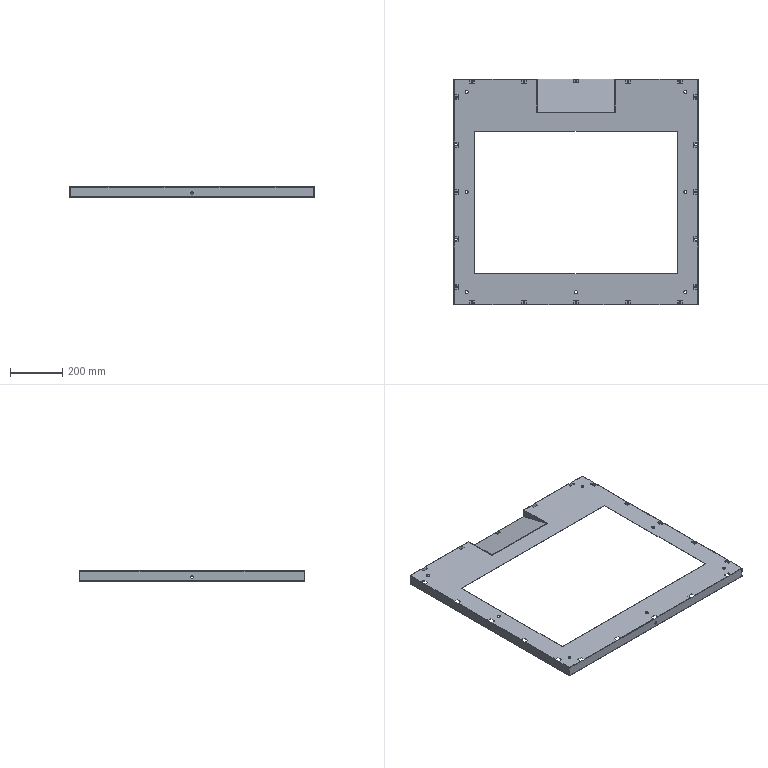Part | 2 solids | 408 faces | box 939 x 869 x 40 mm | volume 604738 mm3 | plane 258 | cylinder 130 | spline 20 | commonest cylinder face diameters 7 x50 0.4 x30 2.4 x30 11 x14 10 x6